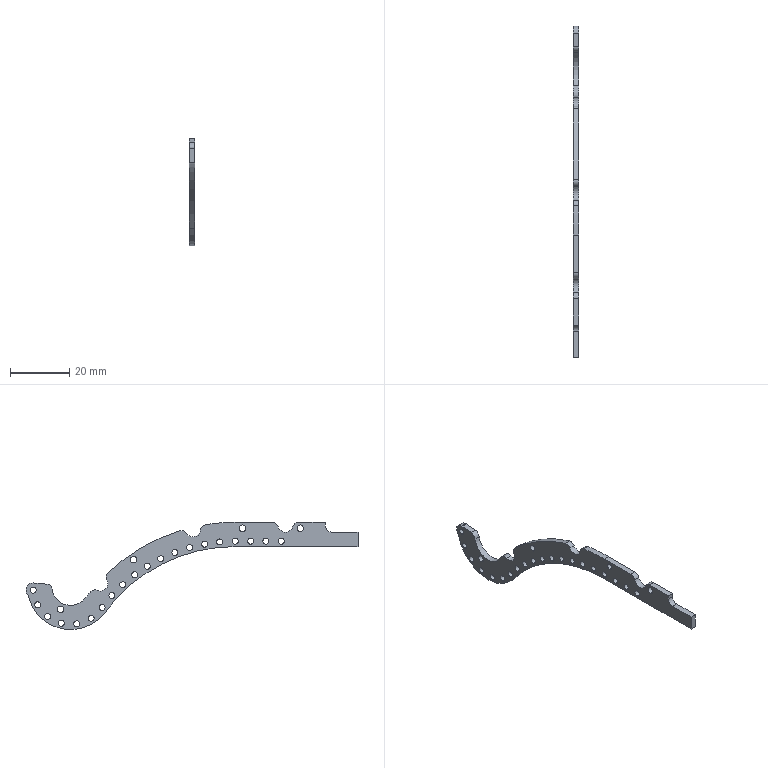Part | SolidWorks | features Extrusion 1, Fillet 1 | 1 solid | 77 faces | box 2 x 112.104 x 36.273 mm | volume 1700 mm3 | cylinder 68 | plane 9 | commonest cylinder face diameters 2.05 x40 4 x9 2.2 x8 5.2 x3 125.4 x3 4.8 x2